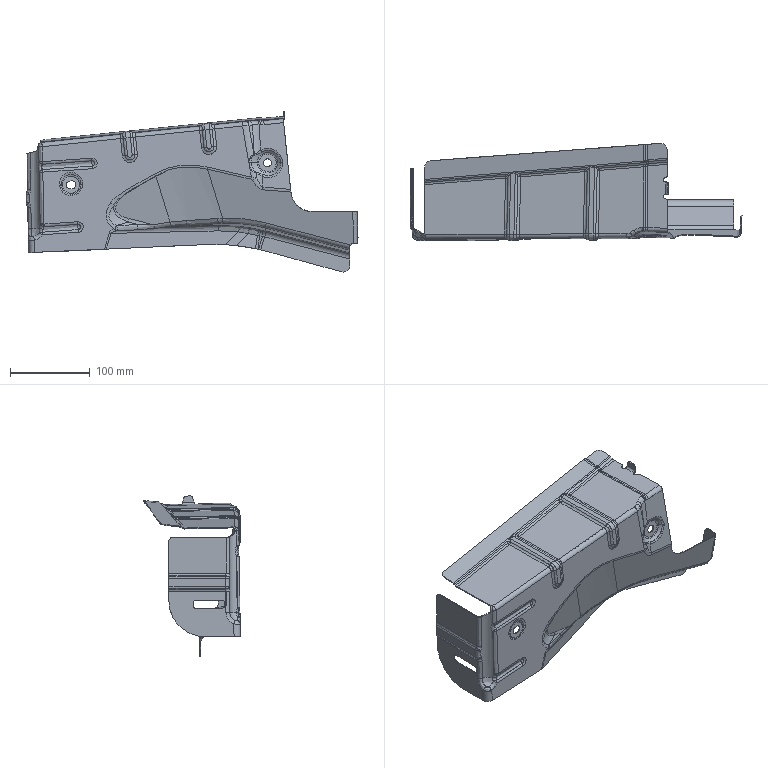Part | 1 solid | 545 faces | box 417.362 x 122.201 x 201.294 mm | volume 122900 mm3 | spline 286 | cylinder 145 | plane 73 | sphere 36 | torus 4 | other 1 | commonest cylinder face diameters 10 x45 7.6 x26 12.4 x17 6 x8 16 x6 13.6 x3